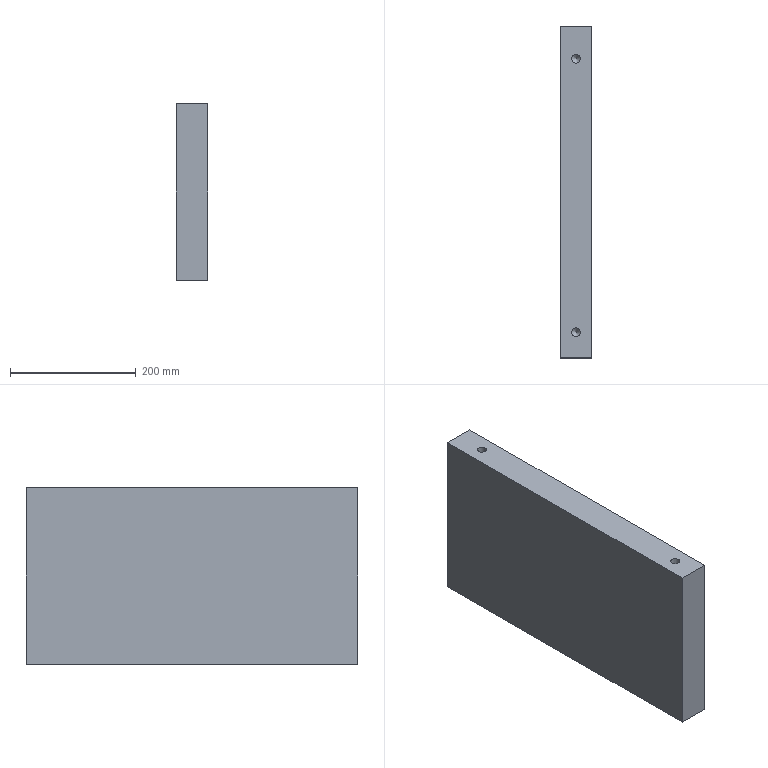Part | NX | features 29 2 | 1 solid | 14 faces | box 50 x 527.5 x 280.5 mm | volume 7373642 mm3 | plane 6 | cylinder 4 | cone 4 | commonest cylinder face diameters 14.1 x4
STEP:
#1=CARTESIAN_POINT('',(627.05,185.5,-493.5));
#2=VERTEX_POINT('',#1);
#3=CARTESIAN_POINT('',(620.,185.5,-493.5));
#4=DIRECTION('',(0.,0.,1.));
#5=DIRECTION('',(1.,0.,0.));
#6=AXIS2_PLACEMENT_3D('',#3,#4,#5);
#7=CIRCLE('',#6,7.05);
#8=EDGE_CURVE('',#2,#2,#7,.T.);
#9=ORIENTED_EDGE('',*,*,#8,.T.);
#10=EDGE_LOOP('',(#9));
#11=FACE_BOUND('',#10,.T.);
#12=CARTESIAN_POINT('',(595.,672.5,-493.5));
#13=VERTEX_POINT('',#12);
#14=CARTESIAN_POINT('',(595.,145.,-493.5));
#15=VERTEX_POINT('',#14);
#16=CARTESIAN_POINT('',(595.,193.,-493.5));
#17=DIRECTION('',(0.,-1.,0.));
#18=VECTOR('',#17,1000.);
#19=LINE('',#16,#18);
#20=EDGE_CURVE('',#13,#15,#19,.T.);
#21=ORIENTED_EDGE('',*,*,#20,.F.);
#22=CARTESIAN_POINT('',(645.,672.5,-493.5));
#23=VERTEX_POINT('',#22);
#24=CARTESIAN_POINT('',(322.5,672.5,-493.5));
#25=DIRECTION('',(1.,0.,0.));
#26=VECTOR('',#25,1000.);
#27=LINE('',#24,#26);
#28=EDGE_CURVE('',#13,#23,#27,.T.);
#29=ORIENTED_EDGE('',*,*,#28,.T.);
#30=CARTESIAN_POINT('',(645.,145.,-493.5));
#31=VERTEX_POINT('',#30);
#32=CARTESIAN_POINT('',(645.,193.,-493.5));
#33=DIRECTION('',(0.,1.,0.));
#34=VECTOR('',#33,1000.);
#35=LINE('',#32,#34);
#36=EDGE_CURVE('',#31,#23,#35,.T.);
#37=ORIENTED_EDGE('',*,*,#36,.F.);
#38=CARTESIAN_POINT('',(845.,145.,-493.5));
#39=DIRECTION('',(-1.,0.,0.));
#40=VECTOR('',#39,1000.);
#41=LINE('',#38,#40);
#42=EDGE_CURVE('',#31,#15,#41,.T.);
#43=ORIENTED_EDGE('',*,*,#42,.T.);
#44=EDGE_LOOP('',(#21,#29,#37,#43));
#45=FACE_BOUND('',#44,.T.);
#46=CARTESIAN_POINT('',(627.05,620.5,-493.5));
#47=VERTEX_POINT('',#46);
#48=CARTESIAN_POINT('',(620.,620.5,-493.5));
#49=DIRECTION('',(0.,0.,1.));
#50=DIRECTION('',(1.,0.,0.));
#51=AXIS2_PLACEMENT_3D('',#48,#49,#50);
#52=CIRCLE('',#51,7.05);
#53=EDGE_CURVE('',#47,#47,#52,.T.);
#54=ORIENTED_EDGE('',*,*,#53,.T.);
#55=EDGE_LOOP('',(#54));
#56=FACE_BOUND('',#55,.T.);
#57=CARTESIAN_POINT('',(1945.,0.,-493.5));
#58=DIRECTION('',(0.,0.,-1.));
#59=DIRECTION('',(1.,0.,0.));
#60=AXIS2_PLACEMENT_3D('',#57,#58,#59);
#61=PLANE('',#60);
#62=ADVANCED_FACE('',(#11,#45,#56),#61,.T.);
#63=CARTESIAN_POINT('',(627.05,185.5,-213.));
#64=VERTEX_POINT('',#63);
#65=CARTESIAN_POINT('',(620.,185.5,-213.));
#66=DIRECTION('',(0.,0.,-1.));
#67=DIRECTION('',(1.,0.,0.));
#68=AXIS2_PLACEMENT_3D('',#65,#66,#67);
#69=CIRCLE('',#68,7.05);
#70=EDGE_CURVE('',#64,#64,#69,.T.);
#71=ORIENTED_EDGE('',*,*,#70,.T.);
#72=EDGE_LOOP('',(#71));
#73=FACE_BOUND('',#72,.T.);
#74=CARTESIAN_POINT('',(645.,672.5,-213.));
#75=VERTEX_POINT('',#74);
#76=CARTESIAN_POINT('',(645.,145.,-213.));
#77=VERTEX_POINT('',#76);
#78=CARTESIAN_POINT('',(645.,193.,-213.));
#79=DIRECTION('',(0.,-1.,0.));
#80=VECTOR('',#79,1000.);
#81=LINE('',#78,#80);
#82=EDGE_CURVE('',#75,#77,#81,.T.);
#83=ORIENTED_EDGE('',*,*,#82,.F.);
#84=CARTESIAN_POINT('',(595.,672.5,-213.));
#85=VERTEX_POINT('',#84);
#86=CARTESIAN_POINT('',(322.5,672.5,-213.));
#87=DIRECTION('',(-1.,0.,0.));
#88=VECTOR('',#87,1000.);
#89=LINE('',#86,#88);
#90=EDGE_CURVE('',#75,#85,#89,.T.);
#91=ORIENTED_EDGE('',*,*,#90,.T.);
#92=CARTESIAN_POINT('',(595.,145.,-213.));
#93=VERTEX_POINT('',#92);
#94=CARTESIAN_POINT('',(595.,193.,-213.));
#95=DIRECTION('',(0.,1.,0.));
#96=VECTOR('',#95,1000.);
#97=LINE('',#94,#96);
#98=EDGE_CURVE('',#93,#85,#97,.T.);
#99=ORIENTED_EDGE('',*,*,#98,.F.);
#100=CARTESIAN_POINT('',(845.,145.,-213.));
#101=DIRECTION('',(1.,0.,0.));
#102=VECTOR('',#101,1000.);
#103=LINE('',#100,#102);
#104=EDGE_CURVE('',#93,#77,#103,.T.);
#105=ORIENTED_EDGE('',*,*,#104,.T.);
#106=EDGE_LOOP('',(#83,#91,#99,#105));
#107=FACE_BOUND('',#106,.T.);
#108=CARTESIAN_POINT('',(627.05,620.5,-213.));
#109=VERTEX_POINT('',#108);
#110=CARTESIAN_POINT('',(620.,620.5,-213.));
#111=DIRECTION('',(0.,0.,-1.));
#112=DIRECTION('',(1.,0.,0.));
#113=AXIS2_PLACEMENT_3D('',#110,#111,#112);
#114=CIRCLE('',#113,7.05);
#115=EDGE_CURVE('',#109,#109,#114,.T.);
#116=ORIENTED_EDGE('',*,*,#115,.T.);
#117=EDGE_LOOP('',(#116));
#118=FACE_BOUND('',#117,.T.);
#119=CARTESIAN_POINT('',(1945.,0.,-213.));
#120=DIRECTION('',(0.,0.,1.));
#121=DIRECTION('',(-1.,0.,0.));
#122=AXIS2_PLACEMENT_3D('',#119,#120,#121);
#123=PLANE('',#122);
#124=ADVANCED_FACE('',(#73,#107,#118),#123,.T.);
#125=CARTESIAN_POINT('',(595.,672.5,91.));
#126=DIRECTION('',(0.,0.,-1.));
#127=VECTOR('',#126,1000.);
#128=LINE('',#125,#127);
#129=EDGE_CURVE('',#85,#13,#128,.T.);
#130=ORIENTED_EDGE('',*,*,#129,.T.);
#131=ORIENTED_EDGE('',*,*,#20,.T.);
#132=CARTESIAN_POINT('',(595.,145.,-2230.5));
#133=DIRECTION('',(0.,0.,1.));
#134=VECTOR('',#133,1000.);
#135=LINE('',#132,#134);
#136=EDGE_CURVE('',#15,#93,#135,.T.);
#137=ORIENTED_EDGE('',*,*,#136,.T.);
#138=ORIENTED_EDGE('',*,*,#98,.T.);
#139=EDGE_LOOP('',(#130,#131,#137,#138));
#140=FACE_BOUND('',#139,.T.);
#141=CARTESIAN_POINT('',(595.,193.,-205.5));
#142=DIRECTION('',(-1.,0.,0.));
#143=DIRECTION('',(0.,0.,1.));
#144=AXIS2_PLACEMENT_3D('',#141,#142,#143);
#145=PLANE('',#144);
#146=ADVANCED_FACE('',(#140),#145,.T.);
#147=CARTESIAN_POINT('',(645.,145.,-205.5));
#148=DIRECTION('',(0.,0.,1.));
#149=VECTOR('',#148,1000.);
#150=LINE('',#147,#149);
#151=EDGE_CURVE('',#31,#77,#150,.T.);
#152=ORIENTED_EDGE('',*,*,#151,.F.);
#153=ORIENTED_EDGE('',*,*,#36,.T.);
#154=CARTESIAN_POINT('',(645.,672.5,-205.5));
#155=DIRECTION('',(0.,0.,-1.));
#156=VECTOR('',#155,1000.);
#157=LINE('',#154,#156);
#158=EDGE_CURVE('',#75,#23,#157,.T.);
#159=ORIENTED_EDGE('',*,*,#158,.F.);
#160=ORIENTED_EDGE('',*,*,#82,.T.);
#161=EDGE_LOOP('',(#152,#153,#159,#160));
#162=FACE_BOUND('',#161,.T.);
#163=CARTESIAN_POINT('',(645.,193.,-205.5));
#164=DIRECTION('',(1.,0.,0.));
#165=DIRECTION('',(0.,0.,-1.));
#166=AXIS2_PLACEMENT_3D('',#163,#164,#165);
#167=PLANE('',#166);
#168=ADVANCED_FACE('',(#162),#167,.T.);
#169=ORIENTED_EDGE('',*,*,#28,.F.);
#170=ORIENTED_EDGE('',*,*,#129,.F.);
#171=ORIENTED_EDGE('',*,*,#90,.F.);
#172=ORIENTED_EDGE('',*,*,#158,.T.);
#173=EDGE_LOOP('',(#169,#170,#171,#172));
#174=FACE_BOUND('',#173,.T.);
#175=CARTESIAN_POINT('',(322.5,672.5,91.));
#176=DIRECTION('',(0.,-1.,0.));
#177=DIRECTION('',(-1.,0.,0.));
#178=AXIS2_PLACEMENT_3D('',#175,#176,#177);
#179=PLANE('',#178);
#180=ADVANCED_FACE('',(#174),#179,.F.);
#181=ORIENTED_EDGE('',*,*,#42,.F.);
#182=ORIENTED_EDGE('',*,*,#151,.T.);
#183=ORIENTED_EDGE('',*,*,#104,.F.);
#184=ORIENTED_EDGE('',*,*,#136,.F.);
#185=EDGE_LOOP('',(#181,#182,#183,#184));
#186=FACE_BOUND('',#185,.T.);
#187=CARTESIAN_POINT('',(845.,145.,-2230.5));
#188=DIRECTION('',(0.,1.,0.));
#189=DIRECTION('',(0.,0.,-1.));
#190=AXIS2_PLACEMENT_3D('',#187,#188,#189);
#191=PLANE('',#190);
#192=ADVANCED_FACE('',(#186),#191,.F.);
#193=CARTESIAN_POINT('',(612.95,185.5,-249.95));
#194=VERTEX_POINT('',#193);
#195=CARTESIAN_POINT('',(620.,185.5,-249.95));
#196=DIRECTION('',(0.,0.,-1.));
#197=DIRECTION('',(-1.,0.,0.));
#198=AXIS2_PLACEMENT_3D('',#195,#196,#197);
#199=CIRCLE('',#198,7.05);
#200=EDGE_CURVE('',#194,#194,#199,.T.);
#201=ORIENTED_EDGE('',*,*,#200,.T.);
#202=EDGE_LOOP('',(#201));
#203=FACE_BOUND('',#202,.T.);
#204=ORIENTED_EDGE('',*,*,#70,.F.);
#205=EDGE_LOOP('',(#204));
#206=FACE_BOUND('',#205,.T.);
#207=CARTESIAN_POINT('',(620.,185.5,-213.));
#208=DIRECTION('',(0.,0.,-1.));
#209=DIRECTION('',(-1.,0.,0.));
#210=AXIS2_PLACEMENT_3D('',#207,#208,#209);
#211=CYLINDRICAL_SURFACE('',#210,7.05);
#212=ADVANCED_FACE('',(#203,#206),#211,.F.);
#213=CARTESIAN_POINT('',(620.,185.5,-257.));
#214=VERTEX_POINT('',#213);
#215=VERTEX_LOOP('',#214);
#216=FACE_BOUND('',#215,.T.);
#217=ORIENTED_EDGE('',*,*,#200,.F.);
#218=EDGE_LOOP('',(#217));
#219=FACE_BOUND('',#218,.T.);
#220=CARTESIAN_POINT('',(620.,185.5,-249.95));
#221=DIRECTION('',(0.,0.,1.));
#222=DIRECTION('',(-1.,0.,0.));
#223=AXIS2_PLACEMENT_3D('',#220,#221,#222);
#224=CONICAL_SURFACE('',#223,7.05,0.7854);
#225=ADVANCED_FACE('',(#216,#219),#224,.F.);
#226=CARTESIAN_POINT('',(612.95,620.5,-249.95));
#227=VERTEX_POINT('',#226);
#228=CARTESIAN_POINT('',(620.,620.5,-249.95));
#229=DIRECTION('',(0.,0.,-1.));
#230=DIRECTION('',(-1.,0.,0.));
#231=AXIS2_PLACEMENT_3D('',#228,#229,#230);
#232=CIRCLE('',#231,7.05);
#233=EDGE_CURVE('',#227,#227,#232,.T.);
#234=ORIENTED_EDGE('',*,*,#233,.T.);
#235=EDGE_LOOP('',(#234));
#236=FACE_BOUND('',#235,.T.);
#237=ORIENTED_EDGE('',*,*,#115,.F.);
#238=EDGE_LOOP('',(#237));
#239=FACE_BOUND('',#238,.T.);
#240=CARTESIAN_POINT('',(620.,620.5,-213.));
#241=DIRECTION('',(0.,0.,-1.));
#242=DIRECTION('',(-1.,0.,0.));
#243=AXIS2_PLACEMENT_3D('',#240,#241,#242);
#244=CYLINDRICAL_SURFACE('',#243,7.05);
#245=ADVANCED_FACE('',(#236,#239),#244,.F.);
#246=CARTESIAN_POINT('',(620.,620.5,-257.));
#247=VERTEX_POINT('',#246);
#248=VERTEX_LOOP('',#247);
#249=FACE_BOUND('',#248,.T.);
#250=ORIENTED_EDGE('',*,*,#233,.F.);
#251=EDGE_LOOP('',(#250));
#252=FACE_BOUND('',#251,.T.);
#253=CARTESIAN_POINT('',(620.,620.5,-249.95));
#254=DIRECTION('',(0.,0.,1.));
#255=DIRECTION('',(-1.,0.,0.));
#256=AXIS2_PLACEMENT_3D('',#253,#254,#255);
#257=CONICAL_SURFACE('',#256,7.05,0.7854);
#258=ADVANCED_FACE('',(#249,#252),#257,.F.);
#259=CARTESIAN_POINT('',(627.05,185.5,-456.55));
#260=VERTEX_POINT('',#259);
#261=CARTESIAN_POINT('',(620.,185.5,-456.55));
#262=DIRECTION('',(0.,0.,1.));
#263=DIRECTION('',(1.,0.,0.));
#264=AXIS2_PLACEMENT_3D('',#261,#262,#263);
#265=CIRCLE('',#264,7.05);
#266=EDGE_CURVE('',#260,#260,#265,.T.);
#267=ORIENTED_EDGE('',*,*,#266,.T.);
#268=EDGE_LOOP('',(#267));
#269=FACE_BOUND('',#268,.T.);
#270=ORIENTED_EDGE('',*,*,#8,.F.);
#271=EDGE_LOOP('',(#270));
#272=FACE_BOUND('',#271,.T.);
#273=CARTESIAN_POINT('',(620.,185.5,-493.5));
#274=DIRECTION('',(0.,0.,1.));
#275=DIRECTION('',(-1.,0.,0.));
#276=AXIS2_PLACEMENT_3D('',#273,#274,#275);
#277=CYLINDRICAL_SURFACE('',#276,7.05);
#278=ADVANCED_FACE('',(#269,#272),#277,.F.);
#279=CARTESIAN_POINT('',(620.,185.5,-449.5));
#280=VERTEX_POINT('',#279);
#281=VERTEX_LOOP('',#280);
#282=FACE_BOUND('',#281,.T.);
#283=ORIENTED_EDGE('',*,*,#266,.F.);
#284=EDGE_LOOP('',(#283));
#285=FACE_BOUND('',#284,.T.);
#286=CARTESIAN_POINT('',(620.,185.5,-456.55));
#287=DIRECTION('',(0.,0.,-1.));
#288=DIRECTION('',(1.,0.,0.));
#289=AXIS2_PLACEMENT_3D('',#286,#287,#288);
#290=CONICAL_SURFACE('',#289,7.05,0.7854);
#291=ADVANCED_FACE('',(#282,#285),#290,.F.);
#292=CARTESIAN_POINT('',(627.05,620.5,-456.55));
#293=VERTEX_POINT('',#292);
#294=CARTESIAN_POINT('',(620.,620.5,-456.55));
#295=DIRECTION('',(0.,0.,1.));
#296=DIRECTION('',(1.,0.,0.));
#297=AXIS2_PLACEMENT_3D('',#294,#295,#296);
#298=CIRCLE('',#297,7.05);
#299=EDGE_CURVE('',#293,#293,#298,.T.);
#300=ORIENTED_EDGE('',*,*,#299,.T.);
#301=EDGE_LOOP('',(#300));
#302=FACE_BOUND('',#301,.T.);
#303=ORIENTED_EDGE('',*,*,#53,.F.);
#304=EDGE_LOOP('',(#303));
#305=FACE_BOUND('',#304,.T.);
#306=CARTESIAN_POINT('',(620.,620.5,-493.5));
#307=DIRECTION('',(0.,0.,1.));
#308=DIRECTION('',(-1.,0.,0.));
#309=AXIS2_PLACEMENT_3D('',#306,#307,#308);
#310=CYLINDRICAL_SURFACE('',#309,7.05);
#311=ADVANCED_FACE('',(#302,#305),#310,.F.);
#312=CARTESIAN_POINT('',(620.,620.5,-449.5));
#313=VERTEX_POINT('',#312);
#314=VERTEX_LOOP('',#313);
#315=FACE_BOUND('',#314,.T.);
#316=ORIENTED_EDGE('',*,*,#299,.F.);
#317=EDGE_LOOP('',(#316));
#318=FACE_BOUND('',#317,.T.);
#319=CARTESIAN_POINT('',(620.,620.5,-456.55));
#320=DIRECTION('',(0.,0.,-1.));
#321=DIRECTION('',(1.,0.,0.));
#322=AXIS2_PLACEMENT_3D('',#319,#320,#321);
#323=CONICAL_SURFACE('',#322,7.05,0.7854);
#324=ADVANCED_FACE('',(#315,#318),#323,.F.);
#325=CLOSED_SHELL('',(#62,#124,#146,#168,#180,#192,#212,#225,#245,#258,#278,#291,#311,#324));
#326=MANIFOLD_SOLID_BREP('',#325);
#327=(LENGTH_UNIT()NAMED_UNIT(*)SI_UNIT(.MILLI.,.METRE.));
#328=UNCERTAINTY_MEASURE_WITH_UNIT(LENGTH_MEASURE(0.00001),#327,'','');
#329=(NAMED_UNIT(*)PLANE_ANGLE_UNIT()SI_UNIT($,.RADIAN.));
#330=(NAMED_UNIT(*)SI_UNIT($,.STERADIAN.)SOLID_ANGLE_UNIT());
#331=(GEOMETRIC_REPRESENTATION_CONTEXT(3)GLOBAL_UNCERTAINTY_ASSIGNED_CONTEXT((#328))GLOBAL_UNIT_ASSIGNED_CONTEXT((#327,#329,#330))REPRESENTATION_CONTEXT('',''));
#332=ADVANCED_BREP_SHAPE_REPRESENTATION('',(#326),#331);